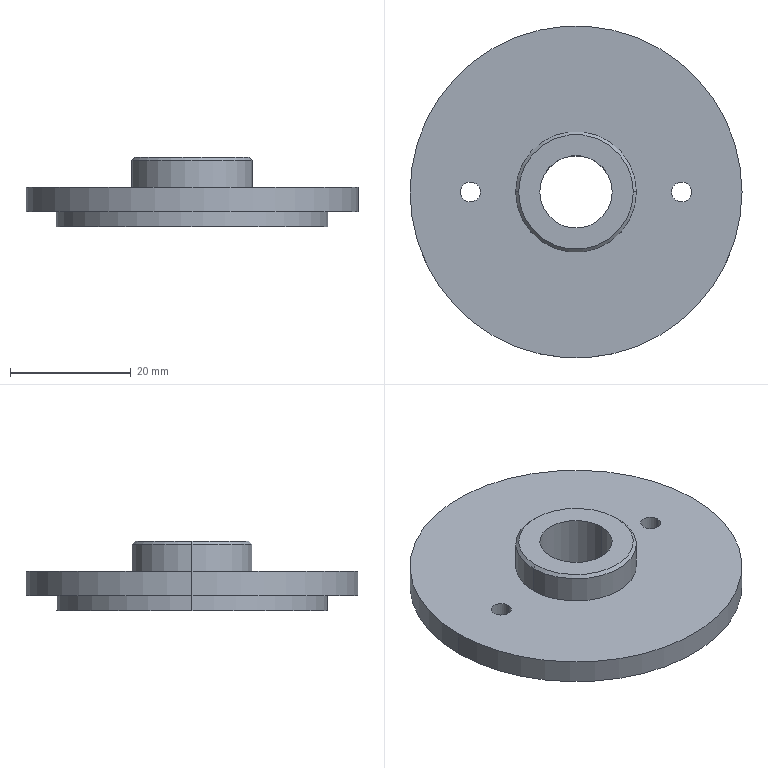Part | STEP file | PN_0098 tensioning part | 1 solid | 18 faces | box 55 x 55 x 11.5 mm | volume 13631 mm3 | cylinder 12 | plane 4 | cone 2 | commonest cylinder face diameters 3.3 x4 12 x2 20 x2 45 x2 55 x2
STEP:
#1=CARTESIAN_POINT('',(0.,0.,0.));
#2=DIRECTION('',(0.,0.,1.));
#3=DIRECTION('',(1.,0.,0.));
#4=AXIS2_PLACEMENT_3D('',#1,#2,#3);
#5=CARTESIAN_POINT('',(9.5,0.,9.));
#6=VERTEX_POINT('',#5);
#7=CARTESIAN_POINT('',(-9.5,0.,9.));
#8=VERTEX_POINT('',#7);
#9=CARTESIAN_POINT('',(0.,0.,9.));
#10=DIRECTION('',(0.,0.,1.));
#11=DIRECTION('',(1.,0.,0.));
#12=AXIS2_PLACEMENT_3D('',#9,#10,#11);
#13=CIRCLE('',#12,9.5);
#14=CARTESIAN_POINT('',(0.,0.,9.));
#15=DIRECTION('',(0.,0.,-1.));
#16=DIRECTION('',(-1.,0.,0.));
#17=AXIS2_PLACEMENT_3D('',#14,#15,#16);
#18=CONICAL_SURFACE('',#17,9.5,0.7854);
#19=CARTESIAN_POINT('',(3.142,0.));
#20=DIRECTION('',(-1.,0.));
#21=VECTOR('',#20,1.);
#22=LINE('',#19,#21);
#23=(GEOMETRIC_REPRESENTATION_CONTEXT(2)PARAMETRIC_REPRESENTATION_CONTEXT()REPRESENTATION_CONTEXT('',''));
#24=DEFINITIONAL_REPRESENTATION('',(#22),#23);
#25=PCURVE('',#18,#24);
#26=CARTESIAN_POINT('',(0.,0.,9.));
#27=DIRECTION('',(0.,0.,1.));
#28=DIRECTION('',(1.,0.,0.));
#29=AXIS2_PLACEMENT_3D('',#26,#27,#28);
#30=PLANE('',#29);
#31=CARTESIAN_POINT('',(0.,0.));
#32=DIRECTION('',(1.,0.));
#33=AXIS2_PLACEMENT_2D('',#31,#32);
#34=CIRCLE('',#33,9.5);
#35=(GEOMETRIC_REPRESENTATION_CONTEXT(2)PARAMETRIC_REPRESENTATION_CONTEXT()REPRESENTATION_CONTEXT('',''));
#36=DEFINITIONAL_REPRESENTATION('',(#34),#35);
#37=PCURVE('',#30,#36);
#38=SURFACE_CURVE('',#13,(#25,#37),.PCURVE_S1.);
#39=EDGE_CURVE('',#6,#8,#38,.T.);
#40=ORIENTED_EDGE('',*,*,#39,.F.);
#41=CARTESIAN_POINT('',(10.,0.,8.5));
#42=VERTEX_POINT('',#41);
#43=CARTESIAN_POINT('',(9.5,0.,9.));
#44=DIRECTION('',(0.7071,0.,-0.7071));
#45=VECTOR('',#44,1.);
#46=LINE('',#43,#45);
#47=CARTESIAN_POINT('',(3.142,0.));
#48=DIRECTION('',(0.,1.));
#49=VECTOR('',#48,1.);
#50=LINE('',#47,#49);
#51=(GEOMETRIC_REPRESENTATION_CONTEXT(2)PARAMETRIC_REPRESENTATION_CONTEXT()REPRESENTATION_CONTEXT('',''));
#52=DEFINITIONAL_REPRESENTATION('',(#50),#51);
#53=PCURVE('',#18,#52);
#54=CARTESIAN_POINT('',(0.,0.,9.));
#55=DIRECTION('',(0.,0.,-1.));
#56=DIRECTION('',(-1.,0.,0.));
#57=AXIS2_PLACEMENT_3D('',#54,#55,#56);
#58=CONICAL_SURFACE('',#57,9.5,0.7854);
#59=CARTESIAN_POINT('',(3.142,0.));
#60=DIRECTION('',(0.,1.));
#61=VECTOR('',#60,1.);
#62=LINE('',#59,#61);
#63=(GEOMETRIC_REPRESENTATION_CONTEXT(2)PARAMETRIC_REPRESENTATION_CONTEXT()REPRESENTATION_CONTEXT('',''));
#64=DEFINITIONAL_REPRESENTATION('',(#62),#63);
#65=PCURVE('',#58,#64);
#66=SURFACE_CURVE('',#46,(#53,#65),.PCURVE_S1.);
#67=EDGE_CURVE('',#6,#42,#66,.T.);
#68=ORIENTED_EDGE('',*,*,#67,.T.);
#69=CARTESIAN_POINT('',(-10.,0.,8.5));
#70=VERTEX_POINT('',#69);
#71=CARTESIAN_POINT('',(0.,0.,8.5));
#72=DIRECTION('',(0.,0.,-1.));
#73=DIRECTION('',(1.,0.,0.));
#74=AXIS2_PLACEMENT_3D('',#71,#72,#73);
#75=CIRCLE('',#74,10.);
#76=CARTESIAN_POINT('',(-3.142,0.5));
#77=DIRECTION('',(1.,0.));
#78=VECTOR('',#77,1.);
#79=LINE('',#76,#78);
#80=(GEOMETRIC_REPRESENTATION_CONTEXT(2)PARAMETRIC_REPRESENTATION_CONTEXT()REPRESENTATION_CONTEXT('',''));
#81=DEFINITIONAL_REPRESENTATION('',(#79),#80);
#82=PCURVE('',#18,#81);
#83=CARTESIAN_POINT('',(0.,0.,9.));
#84=DIRECTION('',(0.,0.,-1.));
#85=DIRECTION('',(-1.,0.,0.));
#86=AXIS2_PLACEMENT_3D('',#83,#84,#85);
#87=CYLINDRICAL_SURFACE('',#86,10.);
#88=CARTESIAN_POINT('',(-3.142,0.5));
#89=DIRECTION('',(1.,0.));
#90=VECTOR('',#89,1.);
#91=LINE('',#88,#90);
#92=(GEOMETRIC_REPRESENTATION_CONTEXT(2)PARAMETRIC_REPRESENTATION_CONTEXT()REPRESENTATION_CONTEXT('',''));
#93=DEFINITIONAL_REPRESENTATION('',(#91),#92);
#94=PCURVE('',#87,#93);
#95=SURFACE_CURVE('',#75,(#82,#94),.PCURVE_S1.);
#96=EDGE_CURVE('',#70,#42,#95,.T.);
#97=ORIENTED_EDGE('',*,*,#96,.F.);
#98=CARTESIAN_POINT('',(-9.5,0.,9.));
#99=DIRECTION('',(-0.7071,0.,-0.7071));
#100=VECTOR('',#99,1.);
#101=LINE('',#98,#100);
#102=CARTESIAN_POINT('',(0.,0.));
#103=DIRECTION('',(0.,1.));
#104=VECTOR('',#103,1.);
#105=LINE('',#102,#104);
#106=(GEOMETRIC_REPRESENTATION_CONTEXT(2)PARAMETRIC_REPRESENTATION_CONTEXT()REPRESENTATION_CONTEXT('',''));
#107=DEFINITIONAL_REPRESENTATION('',(#105),#106);
#108=PCURVE('',#18,#107);
#109=CARTESIAN_POINT('',(6.283,0.));
#110=DIRECTION('',(0.,1.));
#111=VECTOR('',#110,1.);
#112=LINE('',#109,#111);
#113=(GEOMETRIC_REPRESENTATION_CONTEXT(2)PARAMETRIC_REPRESENTATION_CONTEXT()REPRESENTATION_CONTEXT('',''));
#114=DEFINITIONAL_REPRESENTATION('',(#112),#113);
#115=PCURVE('',#58,#114);
#116=SURFACE_CURVE('',#101,(#108,#115),.PCURVE_S1.);
#117=EDGE_CURVE('',#8,#70,#116,.T.);
#118=ORIENTED_EDGE('',*,*,#117,.F.);
#119=EDGE_LOOP('',(#40,#68,#97,#118));
#120=FACE_BOUND('',#119,.T.);
#121=ADVANCED_FACE('',(#120),#18,.T.);
#122=CARTESIAN_POINT('',(-15.85,0.,-2.5));
#123=VERTEX_POINT('',#122);
#124=CARTESIAN_POINT('',(-15.85,0.,4.));
#125=VERTEX_POINT('',#124);
#126=CARTESIAN_POINT('',(-15.85,0.,4.));
#127=DIRECTION('',(0.,0.,1.));
#128=VECTOR('',#127,1.);
#129=LINE('',#126,#128);
#130=CARTESIAN_POINT('',(-17.5,0.,4.));
#131=DIRECTION('',(0.,0.,1.));
#132=DIRECTION('',(1.,0.,0.));
#133=AXIS2_PLACEMENT_3D('',#130,#131,#132);
#134=CYLINDRICAL_SURFACE('',#133,1.65);
#135=CARTESIAN_POINT('',(6.283,0.));
#136=DIRECTION('',(0.,1.));
#137=VECTOR('',#136,1.);
#138=LINE('',#135,#137);
#139=(GEOMETRIC_REPRESENTATION_CONTEXT(2)PARAMETRIC_REPRESENTATION_CONTEXT()REPRESENTATION_CONTEXT('',''));
#140=DEFINITIONAL_REPRESENTATION('',(#138),#139);
#141=PCURVE('',#134,#140);
#142=CARTESIAN_POINT('',(-17.5,0.,4.));
#143=DIRECTION('',(0.,0.,1.));
#144=DIRECTION('',(1.,0.,0.));
#145=AXIS2_PLACEMENT_3D('',#142,#143,#144);
#146=CYLINDRICAL_SURFACE('',#145,1.65);
#147=CARTESIAN_POINT('',(0.,0.));
#148=DIRECTION('',(0.,1.));
#149=VECTOR('',#148,1.);
#150=LINE('',#147,#149);
#151=(GEOMETRIC_REPRESENTATION_CONTEXT(2)PARAMETRIC_REPRESENTATION_CONTEXT()REPRESENTATION_CONTEXT('',''));
#152=DEFINITIONAL_REPRESENTATION('',(#150),#151);
#153=PCURVE('',#146,#152);
#154=SURFACE_CURVE('',#129,(#141,#153),.PCURVE_S1.);
#155=EDGE_CURVE('',#123,#125,#154,.T.);
#156=ORIENTED_EDGE('',*,*,#155,.T.);
#157=CARTESIAN_POINT('',(-19.15,0.,4.));
#158=VERTEX_POINT('',#157);
#159=CARTESIAN_POINT('',(-17.5,0.,4.));
#160=DIRECTION('',(0.,0.,1.));
#161=DIRECTION('',(1.,0.,0.));
#162=AXIS2_PLACEMENT_3D('',#159,#160,#161);
#163=CIRCLE('',#162,1.65);
#164=CARTESIAN_POINT('',(0.,0.));
#165=DIRECTION('',(1.,0.));
#166=VECTOR('',#165,1.);
#167=LINE('',#164,#166);
#168=(GEOMETRIC_REPRESENTATION_CONTEXT(2)PARAMETRIC_REPRESENTATION_CONTEXT()REPRESENTATION_CONTEXT('',''));
#169=DEFINITIONAL_REPRESENTATION('',(#167),#168);
#170=PCURVE('',#134,#169);
#171=CARTESIAN_POINT('',(0.,0.,4.));
#172=DIRECTION('',(0.,0.,1.));
#173=DIRECTION('',(1.,0.,0.));
#174=AXIS2_PLACEMENT_3D('',#171,#172,#173);
#175=PLANE('',#174);
#176=CARTESIAN_POINT('',(-17.5,0.));
#177=DIRECTION('',(1.,0.));
#178=AXIS2_PLACEMENT_2D('',#176,#177);
#179=CIRCLE('',#178,1.65);
#180=(GEOMETRIC_REPRESENTATION_CONTEXT(2)PARAMETRIC_REPRESENTATION_CONTEXT()REPRESENTATION_CONTEXT('',''));
#181=DEFINITIONAL_REPRESENTATION('',(#179),#180);
#182=PCURVE('',#175,#181);
#183=SURFACE_CURVE('',#163,(#170,#182),.PCURVE_S1.);
#184=EDGE_CURVE('',#158,#125,#183,.T.);
#185=ORIENTED_EDGE('',*,*,#184,.F.);
#186=CARTESIAN_POINT('',(-19.15,0.,-2.5));
#187=VERTEX_POINT('',#186);
#188=CARTESIAN_POINT('',(-19.15,0.,4.));
#189=DIRECTION('',(0.,0.,1.));
#190=VECTOR('',#189,1.);
#191=LINE('',#188,#190);
#192=CARTESIAN_POINT('',(3.142,0.));
#193=DIRECTION('',(0.,1.));
#194=VECTOR('',#193,1.);
#195=LINE('',#192,#194);
#196=(GEOMETRIC_REPRESENTATION_CONTEXT(2)PARAMETRIC_REPRESENTATION_CONTEXT()REPRESENTATION_CONTEXT('',''));
#197=DEFINITIONAL_REPRESENTATION('',(#195),#196);
#198=PCURVE('',#134,#197);
#199=CARTESIAN_POINT('',(3.142,0.));
#200=DIRECTION('',(0.,1.));
#201=VECTOR('',#200,1.);
#202=LINE('',#199,#201);
#203=(GEOMETRIC_REPRESENTATION_CONTEXT(2)PARAMETRIC_REPRESENTATION_CONTEXT()REPRESENTATION_CONTEXT('',''));
#204=DEFINITIONAL_REPRESENTATION('',(#202),#203);
#205=PCURVE('',#146,#204);
#206=SURFACE_CURVE('',#191,(#198,#205),.PCURVE_S1.);
#207=EDGE_CURVE('',#187,#158,#206,.T.);
#208=ORIENTED_EDGE('',*,*,#207,.F.);
#209=CARTESIAN_POINT('',(-17.5,0.,-2.5));
#210=DIRECTION('',(0.,0.,1.));
#211=DIRECTION('',(1.,0.,0.));
#212=AXIS2_PLACEMENT_3D('',#209,#210,#211);
#213=CIRCLE('',#212,1.65);
#214=CARTESIAN_POINT('',(0.,-6.5));
#215=DIRECTION('',(1.,0.));
#216=VECTOR('',#215,1.);
#217=LINE('',#214,#216);
#218=(GEOMETRIC_REPRESENTATION_CONTEXT(2)PARAMETRIC_REPRESENTATION_CONTEXT()REPRESENTATION_CONTEXT('',''));
#219=DEFINITIONAL_REPRESENTATION('',(#217),#218);
#220=PCURVE('',#134,#219);
#221=CARTESIAN_POINT('',(0.,0.,-2.5));
#222=DIRECTION('',(0.,0.,-1.));
#223=DIRECTION('',(-1.,0.,0.));
#224=AXIS2_PLACEMENT_3D('',#221,#222,#223);
#225=PLANE('',#224);
#226=CARTESIAN_POINT('',(15.85,0.));
#227=CARTESIAN_POINT('',(15.85,2.858));
#228=CARTESIAN_POINT('',(18.325,1.429));
#229=CARTESIAN_POINT('',(20.8,0.));
#230=CARTESIAN_POINT('',(18.325,-1.429));
#231=CARTESIAN_POINT('',(15.85,-2.858));
#232=CARTESIAN_POINT('',(15.85,0.));
#233=(BOUNDED_CURVE()B_SPLINE_CURVE(2,(#226,#227,#228,#229,#230,#231,#232),.UNSPECIFIED.,.T.,.F.)B_SPLINE_CURVE_WITH_KNOTS((1,2,2,2,2,1),(-2.094,0.,2.094,4.189,6.283,8.378),.UNSPECIFIED.)CURVE()GEOMETRIC_REPRESENTATION_ITEM()RATIONAL_B_SPLINE_CURVE((1.,0.5,1.,0.5,1.,0.5,1.))REPRESENTATION_ITEM(''));
#234=(GEOMETRIC_REPRESENTATION_CONTEXT(2)PARAMETRIC_REPRESENTATION_CONTEXT()REPRESENTATION_CONTEXT('',''));
#235=DEFINITIONAL_REPRESENTATION('',(#233),#234);
#236=PCURVE('',#225,#235);
#237=SURFACE_CURVE('',#213,(#220,#236),.PCURVE_S1.);
#238=EDGE_CURVE('',#187,#123,#237,.T.);
#239=ORIENTED_EDGE('',*,*,#238,.T.);
#240=EDGE_LOOP('',(#156,#185,#208,#239));
#241=FACE_BOUND('',#240,.F.);
#242=ADVANCED_FACE('',(#241),#134,.F.);
#243=CARTESIAN_POINT('',(19.15,0.,-2.5));
#244=VERTEX_POINT('',#243);
#245=CARTESIAN_POINT('',(19.15,0.,4.));
#246=VERTEX_POINT('',#245);
#247=CARTESIAN_POINT('',(19.15,0.,4.));
#248=DIRECTION('',(0.,0.,1.));
#249=VECTOR('',#248,1.);
#250=LINE('',#247,#249);
#251=CARTESIAN_POINT('',(17.5,0.,4.));
#252=DIRECTION('',(0.,0.,1.));
#253=DIRECTION('',(1.,0.,0.));
#254=AXIS2_PLACEMENT_3D('',#251,#252,#253);
#255=CYLINDRICAL_SURFACE('',#254,1.65);
#256=CARTESIAN_POINT('',(6.283,0.));
#257=DIRECTION('',(0.,1.));
#258=VECTOR('',#257,1.);
#259=LINE('',#256,#258);
#260=(GEOMETRIC_REPRESENTATION_CONTEXT(2)PARAMETRIC_REPRESENTATION_CONTEXT()REPRESENTATION_CONTEXT('',''));
#261=DEFINITIONAL_REPRESENTATION('',(#259),#260);
#262=PCURVE('',#255,#261);
#263=CARTESIAN_POINT('',(17.5,0.,4.));
#264=DIRECTION('',(0.,0.,1.));
#265=DIRECTION('',(1.,0.,0.));
#266=AXIS2_PLACEMENT_3D('',#263,#264,#265);
#267=CYLINDRICAL_SURFACE('',#266,1.65);
#268=CARTESIAN_POINT('',(0.,0.));
#269=DIRECTION('',(0.,1.));
#270=VECTOR('',#269,1.);
#271=LINE('',#268,#270);
#272=(GEOMETRIC_REPRESENTATION_CONTEXT(2)PARAMETRIC_REPRESENTATION_CONTEXT()REPRESENTATION_CONTEXT('',''));
#273=DEFINITIONAL_REPRESENTATION('',(#271),#272);
#274=PCURVE('',#267,#273);
#275=SURFACE_CURVE('',#250,(#262,#274),.PCURVE_S1.);
#276=EDGE_CURVE('',#244,#246,#275,.T.);
#277=ORIENTED_EDGE('',*,*,#276,.T.);
#278=CARTESIAN_POINT('',(15.85,0.,4.));
#279=VERTEX_POINT('',#278);
#280=CARTESIAN_POINT('',(17.5,0.,4.));
#281=DIRECTION('',(0.,0.,1.));
#282=DIRECTION('',(1.,0.,0.));
#283=AXIS2_PLACEMENT_3D('',#280,#281,#282);
#284=CIRCLE('',#283,1.65);
#285=CARTESIAN_POINT('',(0.,0.));
#286=DIRECTION('',(1.,0.));
#287=VECTOR('',#286,1.);
#288=LINE('',#285,#287);
#289=(GEOMETRIC_REPRESENTATION_CONTEXT(2)PARAMETRIC_REPRESENTATION_CONTEXT()REPRESENTATION_CONTEXT('',''));
#290=DEFINITIONAL_REPRESENTATION('',(#288),#289);
#291=PCURVE('',#255,#290);
#292=CARTESIAN_POINT('',(17.5,0.));
#293=DIRECTION('',(1.,0.));
#294=AXIS2_PLACEMENT_2D('',#292,#293);
#295=CIRCLE('',#294,1.65);
#296=(GEOMETRIC_REPRESENTATION_CONTEXT(2)PARAMETRIC_REPRESENTATION_CONTEXT()REPRESENTATION_CONTEXT('',''));
#297=DEFINITIONAL_REPRESENTATION('',(#295),#296);
#298=PCURVE('',#175,#297);
#299=SURFACE_CURVE('',#284,(#291,#298),.PCURVE_S1.);
#300=EDGE_CURVE('',#279,#246,#299,.T.);
#301=ORIENTED_EDGE('',*,*,#300,.F.);
#302=CARTESIAN_POINT('',(15.85,0.,-2.5));
#303=VERTEX_POINT('',#302);
#304=CARTESIAN_POINT('',(15.85,0.,4.));
#305=DIRECTION('',(0.,0.,1.));
#306=VECTOR('',#305,1.);
#307=LINE('',#304,#306);
#308=CARTESIAN_POINT('',(3.142,0.));
#309=DIRECTION('',(0.,1.));
#310=VECTOR('',#309,1.);
#311=LINE('',#308,#310);
#312=(GEOMETRIC_REPRESENTATION_CONTEXT(2)PARAMETRIC_REPRESENTATION_CONTEXT()REPRESENTATION_CONTEXT('',''));
#313=DEFINITIONAL_REPRESENTATION('',(#311),#312);
#314=PCURVE('',#255,#313);
#315=CARTESIAN_POINT('',(3.142,0.));
#316=DIRECTION('',(0.,1.));
#317=VECTOR('',#316,1.);
#318=LINE('',#315,#317);
#319=(GEOMETRIC_REPRESENTATION_CONTEXT(2)PARAMETRIC_REPRESENTATION_CONTEXT()REPRESENTATION_CONTEXT('',''));
#320=DEFINITIONAL_REPRESENTATION('',(#318),#319);
#321=PCURVE('',#267,#320);
#322=SURFACE_CURVE('',#307,(#314,#321),.PCURVE_S1.);
#323=EDGE_CURVE('',#303,#279,#322,.T.);
#324=ORIENTED_EDGE('',*,*,#323,.F.);
#325=CARTESIAN_POINT('',(17.5,0.,-2.5));
#326=DIRECTION('',(0.,0.,1.));
#327=DIRECTION('',(1.,0.,0.));
#328=AXIS2_PLACEMENT_3D('',#325,#326,#327);
#329=CIRCLE('',#328,1.65);
#330=CARTESIAN_POINT('',(0.,-6.5));
#331=DIRECTION('',(1.,0.));
#332=VECTOR('',#331,1.);
#333=LINE('',#330,#332);
#334=(GEOMETRIC_REPRESENTATION_CONTEXT(2)PARAMETRIC_REPRESENTATION_CONTEXT()REPRESENTATION_CONTEXT('',''));
#335=DEFINITIONAL_REPRESENTATION('',(#333),#334);
#336=PCURVE('',#255,#335);
#337=CARTESIAN_POINT('',(-19.15,0.));
#338=CARTESIAN_POINT('',(-19.15,2.858));
#339=CARTESIAN_POINT('',(-16.675,1.429));
#340=CARTESIAN_POINT('',(-14.2,0.));
#341=CARTESIAN_POINT('',(-16.675,-1.429));
#342=CARTESIAN_POINT('',(-19.15,-2.858));
#343=CARTESIAN_POINT('',(-19.15,0.));
#344=(BOUNDED_CURVE()B_SPLINE_CURVE(2,(#337,#338,#339,#340,#341,#342,#343),.UNSPECIFIED.,.T.,.F.)B_SPLINE_CURVE_WITH_KNOTS((1,2,2,2,2,1),(-2.094,0.,2.094,4.189,6.283,8.378),.UNSPECIFIED.)CURVE()GEOMETRIC_REPRESENTATION_ITEM()RATIONAL_B_SPLINE_CURVE((1.,0.5,1.,0.5,1.,0.5,1.))REPRESENTATION_ITEM(''));
#345=(GEOMETRIC_REPRESENTATION_CONTEXT(2)PARAMETRIC_REPRESENTATION_CONTEXT()REPRESENTATION_CONTEXT('',''));
#346=DEFINITIONAL_REPRESENTATION('',(#344),#345);
#347=PCURVE('',#225,#346);
#348=SURFACE_CURVE('',#329,(#336,#347),.PCURVE_S1.);
#349=EDGE_CURVE('',#303,#244,#348,.T.);
#350=ORIENTED_EDGE('',*,*,#349,.T.);
#351=EDGE_LOOP('',(#277,#301,#324,#350));
#352=FACE_BOUND('',#351,.F.);
#353=ADVANCED_FACE('',(#352),#255,.F.);
#354=CARTESIAN_POINT('',(-22.5,0.,-2.5));
#355=VERTEX_POINT('',#354);
#356=CARTESIAN_POINT('',(22.5,0.,-2.5));
#357=VERTEX_POINT('',#356);
#358=CARTESIAN_POINT('',(0.,0.,-2.5));
#359=DIRECTION('',(0.,0.,-1.));
#360=DIRECTION('',(-1.,0.,0.));
#361=AXIS2_PLACEMENT_3D('',#358,#359,#360);
#362=CIRCLE('',#361,22.5);
#363=CARTESIAN_POINT('',(0.,0.,-2.5));
#364=DIRECTION('',(0.,0.,1.));
#365=DIRECTION('',(1.,0.,0.));
#366=AXIS2_PLACEMENT_3D('',#363,#364,#365);
#367=CYLINDRICAL_SURFACE('',#366,22.5);
#368=CARTESIAN_POINT('',(3.142,0.));
#369=DIRECTION('',(-1.,0.));
#370=VECTOR('',#369,1.);
#371=LINE('',#368,#370);
#372=(GEOMETRIC_REPRESENTATION_CONTEXT(2)PARAMETRIC_REPRESENTATION_CONTEXT()REPRESENTATION_CONTEXT('',''));
#373=DEFINITIONAL_REPRESENTATION('',(#371),#372);
#374=PCURVE('',#367,#373);
#375=CARTESIAN_POINT('',(0.,0.));
#376=DIRECTION('',(1.,0.));
#377=AXIS2_PLACEMENT_2D('',#375,#376);
#378=CIRCLE('',#377,22.5);
#379=(GEOMETRIC_REPRESENTATION_CONTEXT(2)PARAMETRIC_REPRESENTATION_CONTEXT()REPRESENTATION_CONTEXT('',''));
#380=DEFINITIONAL_REPRESENTATION('',(#378),#379);
#381=PCURVE('',#225,#380);
#382=SURFACE_CURVE('',#362,(#374,#381),.PCURVE_S1.);
#383=EDGE_CURVE('',#355,#357,#382,.T.);
#384=ORIENTED_EDGE('',*,*,#383,.F.);
#385=CARTESIAN_POINT('',(-22.5,0.,0.));
#386=VERTEX_POINT('',#385);
#387=CARTESIAN_POINT('',(-22.5,0.,-2.5));
#388=DIRECTION('',(0.,0.,1.));
#389=VECTOR('',#388,1.);
#390=LINE('',#387,#389);
#391=CARTESIAN_POINT('',(3.142,0.));
#392=DIRECTION('',(0.,1.));
#393=VECTOR('',#392,1.);
#394=LINE('',#391,#393);
#395=(GEOMETRIC_REPRESENTATION_CONTEXT(2)PARAMETRIC_REPRESENTATION_CONTEXT()REPRESENTATION_CONTEXT('',''));
#396=DEFINITIONAL_REPRESENTATION('',(#394),#395);
#397=PCURVE('',#367,#396);
#398=CARTESIAN_POINT('',(0.,0.,-2.5));
#399=DIRECTION('',(0.,0.,1.));
#400=DIRECTION('',(1.,0.,0.));
#401=AXIS2_PLACEMENT_3D('',#398,#399,#400);
#402=CYLINDRICAL_SURFACE('',#401,22.5);
#403=CARTESIAN_POINT('',(3.142,0.));
#404=DIRECTION('',(0.,1.));
#405=VECTOR('',#404,1.);
#406=LINE('',#403,#405);
#407=(GEOMETRIC_REPRESENTATION_CONTEXT(2)PARAMETRIC_REPRESENTATION_CONTEXT()REPRESENTATION_CONTEXT('',''));
#408=DEFINITIONAL_REPRESENTATION('',(#406),#407);
#409=PCURVE('',#402,#408);
#410=SURFACE_CURVE('',#390,(#397,#409),.PCURVE_S1.);
#411=EDGE_CURVE('',#355,#386,#410,.T.);
#412=ORIENTED_EDGE('',*,*,#411,.T.);
#413=CARTESIAN_POINT('',(22.5,0.,0.));
#414=VERTEX_POINT('',#413);
#415=CARTESIAN_POINT('',(0.,0.,0.));
#416=DIRECTION('',(0.,0.,-1.));
#417=DIRECTION('',(1.,0.,0.));
#418=AXIS2_PLACEMENT_3D('',#415,#416,#417);
#419=CIRCLE('',#418,22.5);
#420=CARTESIAN_POINT('',(6.283,2.5));
#421=DIRECTION('',(-1.,0.));
#422=VECTOR('',#421,1.);
#423=LINE('',#420,#422);
#424=(GEOMETRIC_REPRESENTATION_CONTEXT(2)PARAMETRIC_REPRESENTATION_CONTEXT()REPRESENTATION_CONTEXT('',''));
#425=DEFINITIONAL_REPRESENTATION('',(#423),#424);
#426=PCURVE('',#367,#425);
#427=CARTESIAN_POINT('',(0.,0.,0.));
#428=DIRECTION('',(0.,0.,1.));
#429=DIRECTION('',(1.,0.,0.));
#430=AXIS2_PLACEMENT_3D('',#427,#428,#429);
#431=PLANE('',#430);
#432=CARTESIAN_POINT('',(22.5,0.));
#433=CARTESIAN_POINT('',(22.5,-38.971));
#434=CARTESIAN_POINT('',(-11.25,-19.486));
#435=CARTESIAN_POINT('',(-45.,0.));
#436=CARTESIAN_POINT('',(-11.25,19.486));
#437=CARTESIAN_POINT('',(22.5,38.971));
#438=CARTESIAN_POINT('',(22.5,0.));
#439=(BOUNDED_CURVE()B_SPLINE_CURVE(2,(#432,#433,#434,#435,#436,#437,#438),.UNSPECIFIED.,.T.,.F.)B_SPLINE_CURVE_WITH_KNOTS((1,2,2,2,2,1),(-2.094,0.,2.094,4.189,6.283,8.378),.UNSPECIFIED.)CURVE()GEOMETRIC_REPRESENTATION_ITEM()RATIONAL_B_SPLINE_CURVE((1.,0.5,1.,0.5,1.,0.5,1.))REPRESENTATION_ITEM(''));
#440=(GEOMETRIC_REPRESENTATION_CONTEXT(2)PARAMETRIC_REPRESENTATION_CONTEXT()REPRESENTATION_CONTEXT('',''));
#441=DEFINITIONAL_REPRESENTATION('',(#439),#440);
#442=PCURVE('',#431,#441);
#443=SURFACE_CURVE('',#419,(#426,#442),.PCURVE_S1.);
#444=EDGE_CURVE('',#386,#414,#443,.T.);
#445=ORIENTED_EDGE('',*,*,#444,.T.);
#446=CARTESIAN_POINT('',(22.5,0.,-2.5));
#447=DIRECTION('',(0.,0.,1.));
#448=VECTOR('',#447,1.);
#449=LINE('',#446,#448);
#450=CARTESIAN_POINT('',(0.,0.));
#451=DIRECTION('',(0.,1.));
#452=VECTOR('',#451,1.);
#453=LINE('',#450,#452);
#454=(GEOMETRIC_REPRESENTATION_CONTEXT(2)PARAMETRIC_REPRESENTATION_CONTEXT()REPRESENTATION_CONTEXT('',''));
#455=DEFINITIONAL_REPRESENTATION('',(#453),#454);
#456=PCURVE('',#367,#455);
#457=CARTESIAN_POINT('',(6.283,0.));
#458=DIRECTION('',(0.,1.));
#459=VECTOR('',#458,1.);
#460=LINE('',#457,#459);
#461=(GEOMETRIC_REPRESENTATION_CONTEXT(2)PARAMETRIC_REPRESENTATION_CONTEXT()REPRESENTATION_CONTEXT('',''));
#462=DEFINITIONAL_REPRESENTATION('',(#460),#461);
#463=PCURVE('',#402,#462);
#464=SURFACE_CURVE('',#449,(#456,#463),.PCURVE_S1.);
#465=EDGE_CURVE('',#357,#414,#464,.T.);
#466=ORIENTED_EDGE('',*,*,#465,.F.);
#467=EDGE_LOOP('',(#384,#412,#445,#466));
#468=FACE_BOUND('',#467,.T.);
#469=ADVANCED_FACE('',(#468),#367,.T.);
#470=ORIENTED_EDGE('',*,*,#96,.T.);
#471=CARTESIAN_POINT('',(10.,0.,4.));
#472=VERTEX_POINT('',#471);
#473=CARTESIAN_POINT('',(10.,0.,9.));
#474=DIRECTION('',(0.,0.,-1.));
#475=VECTOR('',#474,1.);
#476=LINE('',#473,#475);
#477=CARTESIAN_POINT('',(3.142,0.));
#478=DIRECTION('',(0.,1.));
#479=VECTOR('',#478,1.);
#480=LINE('',#477,#479);
#481=(GEOMETRIC_REPRESENTATION_CONTEXT(2)PARAMETRIC_REPRESENTATION_CONTEXT()REPRESENTATION_CONTEXT('',''));
#482=DEFINITIONAL_REPRESENTATION('',(#480),#481);
#483=PCURVE('',#87,#482);
#484=CARTESIAN_POINT('',(0.,0.,9.));
#485=DIRECTION('',(0.,0.,-1.));
#486=DIRECTION('',(-1.,0.,0.));
#487=AXIS2_PLACEMENT_3D('',#484,#485,#486);
#488=CYLINDRICAL_SURFACE('',#487,10.);
#489=CARTESIAN_POINT('',(3.142,0.));
#490=DIRECTION('',(0.,1.));
#491=VECTOR('',#490,1.);
#492=LINE('',#489,#491);
#493=(GEOMETRIC_REPRESENTATION_CONTEXT(2)PARAMETRIC_REPRESENTATION_CONTEXT()REPRESENTATION_CONTEXT('',''));
#494=DEFINITIONAL_REPRESENTATION('',(#492),#493);
#495=PCURVE('',#488,#494);
#496=SURFACE_CURVE('',#476,(#483,#495),.PCURVE_S1.);
#497=EDGE_CURVE('',#42,#472,#496,.T.);
#498=ORIENTED_EDGE('',*,*,#497,.T.);
#499=CARTESIAN_POINT('',(-10.,0.,4.));
#500=VERTEX_POINT('',#499);
#501=CARTESIAN_POINT('',(0.,0.,4.));
#502=DIRECTION('',(0.,0.,1.));
#503=DIRECTION('',(1.,0.,0.));
#504=AXIS2_PLACEMENT_3D('',#501,#502,#503);
#505=CIRCLE('',#504,10.);
#506=CARTESIAN_POINT('',(3.142,5.));
#507=DIRECTION('',(-1.,0.));
#508=VECTOR('',#507,1.);
#509=LINE('',#506,#508);
#510=(GEOMETRIC_REPRESENTATION_CONTEXT(2)PARAMETRIC_REPRESENTATION_CONTEXT()REPRESENTATION_CONTEXT('',''));
#511=DEFINITIONAL_REPRESENTATION('',(#509),#510);
#512=PCURVE('',#87,#511);
#513=CARTESIAN_POINT('',(0.,0.));
#514=DIRECTION('',(1.,0.));
#515=AXIS2_PLACEMENT_2D('',#513,#514);
#516=CIRCLE('',#515,10.);
#517=(GEOMETRIC_REPRESENTATION_CONTEXT(2)PARAMETRIC_REPRESENTATION_CONTEXT()REPRESENTATION_CONTEXT('',''));
#518=DEFINITIONAL_REPRESENTATION('',(#516),#517);
#519=PCURVE('',#175,#518);
#520=SURFACE_CURVE('',#505,(#512,#519),.PCURVE_S1.);
#521=EDGE_CURVE('',#472,#500,#520,.T.);
#522=ORIENTED_EDGE('',*,*,#521,.T.);
#523=CARTESIAN_POINT('',(-10.,0.,9.));
#524=DIRECTION('',(0.,0.,-1.));
#525=VECTOR('',#524,1.);
#526=LINE('',#523,#525);
#527=CARTESIAN_POINT('',(0.,0.));
#528=DIRECTION('',(0.,1.));
#529=VECTOR('',#528,1.);
#530=LINE('',#527,#529);
#531=(GEOMETRIC_REPRESENTATION_CONTEXT(2)PARAMETRIC_REPRESENTATION_CONTEXT()REPRESENTATION_CONTEXT('',''));
#532=DEFINITIONAL_REPRESENTATION('',(#530),#531);
#533=PCURVE('',#87,#532);
#534=CARTESIAN_POINT('',(6.283,0.));
#535=DIRECTION('',(0.,1.));
#536=VECTOR('',#535,1.);
#537=LINE('',#534,#536);
#538=(GEOMETRIC_REPRESENTATION_CONTEXT(2)PARAMETRIC_REPRESENTATION_CONTEXT()REPRESENTATION_CONTEXT('',''));
#539=DEFINITIONAL_REPRESENTATION('',(#537),#538);
#540=PCURVE('',#488,#539);
#541=SURFACE_CURVE('',#526,(#533,#540),.PCURVE_S1.);
#542=EDGE_CURVE('',#70,#500,#541,.T.);
#543=ORIENTED_EDGE('',*,*,#542,.F.);
#544=EDGE_LOOP('',(#470,#498,#522,#543));
#545=FACE_BOUND('',#544,.T.);
#546=ADVANCED_FACE('',(#545),#87,.T.);
#547=CARTESIAN_POINT('',(-6.,0.,9.));
#548=VERTEX_POINT('',#547);
#549=CARTESIAN_POINT('',(-6.,0.,-2.5));
#550=VERTEX_POINT('',#549);
#551=CARTESIAN_POINT('',(-6.,0.,4.));
#552=DIRECTION('',(0.,0.,-1.));
#553=VECTOR('',#552,1.);
#554=LINE('',#551,#553);
#555=CARTESIAN_POINT('',(0.,0.,4.));
#556=DIRECTION('',(0.,0.,-1.));
#557=DIRECTION('',(-1.,0.,0.));
#558=AXIS2_PLACEMENT_3D('',#555,#556,#557);
#559=CYLINDRICAL_SURFACE('',#558,6.);
#560=CARTESIAN_POINT('',(6.283,0.));
#561=DIRECTION('',(0.,1.));
#562=VECTOR('',#561,1.);
#563=LINE('',#560,#562);
#564=(GEOMETRIC_REPRESENTATION_CONTEXT(2)PARAMETRIC_REPRESENTATION_CONTEXT()REPRESENTATION_CONTEXT('',''));
#565=DEFINITIONAL_REPRESENTATION('',(#563),#564);
#566=PCURVE('',#559,#565);
#567=CARTESIAN_POINT('',(0.,0.,4.));
#568=DIRECTION('',(0.,0.,-1.));
#569=DIRECTION('',(-1.,0.,0.));
#570=AXIS2_PLACEMENT_3D('',#567,#568,#569);
#571=CYLINDRICAL_SURFACE('',#570,6.);
#572=CARTESIAN_POINT('',(0.,0.));
#573=DIRECTION('',(0.,1.));
#574=VECTOR('',#573,1.);
#575=LINE('',#572,#574);
#576=(GEOMETRIC_REPRESENTATION_CONTEXT(2)PARAMETRIC_REPRESENTATION_CONTEXT()REPRESENTATION_CONTEXT('',''));
#577=DEFINITIONAL_REPRESENTATION('',(#575),#576);
#578=PCURVE('',#571,#577);
#579=SURFACE_CURVE('',#554,(#566,#578),.PCURVE_S1.);
#580=EDGE_CURVE('',#548,#550,#579,.T.);
#581=ORIENTED_EDGE('',*,*,#580,.T.);
#582=CARTESIAN_POINT('',(6.,0.,-2.5));
#583=VERTEX_POINT('',#582);
#584=CARTESIAN_POINT('',(0.,0.,-2.5));
#585=DIRECTION('',(0.,0.,-1.));
#586=DIRECTION('',(-1.,0.,0.));
#587=AXIS2_PLACEMENT_3D('',#584,#585,#586);
#588=CIRCLE('',#587,6.);
#589=CARTESIAN_POINT('',(0.,6.5));
#590=DIRECTION('',(1.,0.));
#591=VECTOR('',#590,1.);
#592=LINE('',#589,#591);
#593=(GEOMETRIC_REPRESENTATION_CONTEXT(2)PARAMETRIC_REPRESENTATION_CONTEXT()REPRESENTATION_CONTEXT('',''));
#594=DEFINITIONAL_REPRESENTATION('',(#592),#593);
#595=PCURVE('',#559,#594);
#596=CARTESIAN_POINT('',(0.,0.));
#597=DIRECTION('',(1.,0.));
#598=AXIS2_PLACEMENT_2D('',#596,#597);
#599=CIRCLE('',#598,6.);
#600=(GEOMETRIC_REPRESENTATION_CONTEXT(2)PARAMETRIC_REPRESENTATION_CONTEXT()REPRESENTATION_CONTEXT('',''));
#601=DEFINITIONAL_REPRESENTATION('',(#599),#600);
#602=PCURVE('',#225,#601);
#603=SURFACE_CURVE('',#588,(#595,#602),.PCURVE_S1.);
#604=EDGE_CURVE('',#583,#550,#603,.T.);
#605=ORIENTED_EDGE('',*,*,#604,.F.);
#606=CARTESIAN_POINT('',(6.,0.,9.));
#607=VERTEX_POINT('',#606);
#608=CARTESIAN_POINT('',(6.,0.,4.));
#609=DIRECTION('',(0.,0.,-1.));
#610=VECTOR('',#609,1.);
#611=LINE('',#608,#610);
#612=CARTESIAN_POINT('',(3.142,0.));
#613=DIRECTION('',(0.,1.));
#614=VECTOR('',#613,1.);
#615=LINE('',#612,#614);
#616=(GEOMETRIC_REPRESENTATION_CONTEXT(2)PARAMETRIC_REPRESENTATION_CONTEXT()REPRESENTATION_CONTEXT('',''));
#617=DEFINITIONAL_REPRESENTATION('',(#615),#616);
#618=PCURVE('',#559,#617);
#619=CARTESIAN_POINT('',(3.142,0.));
#620=DIRECTION('',(0.,1.));
#621=VECTOR('',#620,1.);
#622=LINE('',#619,#621);
#623=(GEOMETRIC_REPRESENTATION_CONTEXT(2)PARAMETRIC_REPRESENTATION_CONTEXT()REPRESENTATION_CONTEXT('',''));
#624=DEFINITIONAL_REPRESENTATION('',(#622),#623);
#625=PCURVE('',#571,#624);
#626=SURFACE_CURVE('',#611,(#618,#625),.PCURVE_S1.);
#627=EDGE_CURVE('',#607,#583,#626,.T.);
#628=ORIENTED_EDGE('',*,*,#627,.F.);
#629=CARTESIAN_POINT('',(0.,0.,9.));
#630=DIRECTION('',(0.,0.,1.));
#631=DIRECTION('',(1.,0.,0.));
#632=AXIS2_PLACEMENT_3D('',#629,#630,#631);
#633=CIRCLE('',#632,6.);
#634=CARTESIAN_POINT('',(9.425,-5.));
#635=DIRECTION('',(-1.,0.));
#636=VECTOR('',#635,1.);
#637=LINE('',#634,#636);
#638=(GEOMETRIC_REPRESENTATION_CONTEXT(2)PARAMETRIC_REPRESENTATION_CONTEXT()REPRESENTATION_CONTEXT('',''));
#639=DEFINITIONAL_REPRESENTATION('',(#637),#638);
#640=PCURVE('',#559,#639);
#641=CARTESIAN_POINT('',(0.,0.));
#642=DIRECTION('',(1.,0.));
#643=AXIS2_PLACEMENT_2D('',#641,#642);
#644=CIRCLE('',#643,6.);
#645=(GEOMETRIC_REPRESENTATION_CONTEXT(2)PARAMETRIC_REPRESENTATION_CONTEXT()REPRESENTATION_CONTEXT('',''));
#646=DEFINITIONAL_REPRESENTATION('',(#644),#645);
#647=PCURVE('',#30,#646);
#648=SURFACE_CURVE('',#633,(#640,#647),.PCURVE_S1.);
#649=EDGE_CURVE('',#548,#607,#648,.T.);
#650=ORIENTED_EDGE('',*,*,#649,.F.);
#651=EDGE_LOOP('',(#581,#605,#628,#650));
#652=FACE_BOUND('',#651,.F.);
#653=ADVANCED_FACE('',(#652),#559,.F.);
#654=CARTESIAN_POINT('',(27.5,0.,4.));
#655=VERTEX_POINT('',#654);
#656=CARTESIAN_POINT('',(-27.5,0.,4.));
#657=VERTEX_POINT('',#656);
#658=CARTESIAN_POINT('',(0.,0.,4.));
#659=DIRECTION('',(0.,0.,1.));
#660=DIRECTION('',(1.,0.,0.));
#661=AXIS2_PLACEMENT_3D('',#658,#659,#660);
#662=CIRCLE('',#661,27.5);
#663=CARTESIAN_POINT('',(0.,0.,4.));
#664=DIRECTION('',(0.,0.,-1.));
#665=DIRECTION('',(-1.,0.,0.));
#666=AXIS2_PLACEMENT_3D('',#663,#664,#665);
#667=CYLINDRICAL_SURFACE('',#666,27.5);
#668=CARTESIAN_POINT('',(3.142,0.));
#669=DIRECTION('',(-1.,0.));
#670=VECTOR('',#669,1.);
#671=LINE('',#668,#670);
#672=(GEOMETRIC_REPRESENTATION_CONTEXT(2)PARAMETRIC_REPRESENTATION_CONTEXT()REPRESENTATION_CONTEXT('',''));
#673=DEFINITIONAL_REPRESENTATION('',(#671),#672);
#674=PCURVE('',#667,#673);
#675=CARTESIAN_POINT('',(0.,0.));
#676=DIRECTION('',(1.,0.));
#677=AXIS2_PLACEMENT_2D('',#675,#676);
#678=CIRCLE('',#677,27.5);
#679=(GEOMETRIC_REPRESENTATION_CONTEXT(2)PARAMETRIC_REPRESENTATION_CONTEXT()REPRESENTATION_CONTEXT('',''));
#680=DEFINITIONAL_REPRESENTATION('',(#678),#679);
#681=PCURVE('',#175,#680);
#682=SURFACE_CURVE('',#662,(#674,#681),.PCURVE_S1.);
#683=EDGE_CURVE('',#655,#657,#682,.T.);
#684=ORIENTED_EDGE('',*,*,#683,.F.);
#685=CARTESIAN_POINT('',(27.5,0.,0.));
#686=VERTEX_POINT('',#685);
#687=CARTESIAN_POINT('',(27.5,0.,4.));
#688=DIRECTION('',(0.,0.,-1.));
#689=VECTOR('',#688,1.);
#690=LINE('',#687,#689);
#691=CARTESIAN_POINT('',(3.142,0.));
#692=DIRECTION('',(0.,1.));
#693=VECTOR('',#692,1.);
#694=LINE('',#691,#693);
#695=(GEOMETRIC_REPRESENTATION_CONTEXT(2)PARAMETRIC_REPRESENTATION_CONTEXT()REPRESENTATION_CONTEXT('',''));
#696=DEFINITIONAL_REPRESENTATION('',(#694),#695);
#697=PCURVE('',#667,#696);
#698=CARTESIAN_POINT('',(0.,0.,4.));
#699=DIRECTION('',(0.,0.,-1.));
#700=DIRECTION('',(-1.,0.,0.));
#701=AXIS2_PLACEMENT_3D('',#698,#699,#700);
#702=CYLINDRICAL_SURFACE('',#701,27.5);
#703=CARTESIAN_POINT('',(3.142,0.));
#704=DIRECTION('',(0.,1.));
#705=VECTOR('',#704,1.);
#706=LINE('',#703,#705);
#707=(GEOMETRIC_REPRESENTATION_CONTEXT(2)PARAMETRIC_REPRESENTATION_CONTEXT()REPRESENTATION_CONTEXT('',''));
#708=DEFINITIONAL_REPRESENTATION('',(#706),#707);
#709=PCURVE('',#702,#708);
#710=SURFACE_CURVE('',#690,(#697,#709),.PCURVE_S1.);
#711=EDGE_CURVE('',#655,#686,#710,.T.);
#712=ORIENTED_EDGE('',*,*,#711,.T.);
#713=CARTESIAN_POINT('',(-27.5,0.,0.));
#714=VERTEX_POINT('',#713);
#715=CARTESIAN_POINT('',(0.,0.,0.));
#716=DIRECTION('',(0.,0.,1.));
#717=DIRECTION('',(1.,0.,0.));
#718=AXIS2_PLACEMENT_3D('',#715,#716,#717);
#719=CIRCLE('',#718,27.5);
#720=CARTESIAN_POINT('',(3.142,4.));
#721=DIRECTION('',(-1.,0.));
#722=VECTOR('',#721,1.);
#723=LINE('',#720,#722);
#724=(GEOMETRIC_REPRESENTATION_CONTEXT(2)PARAMETRIC_REPRESENTATION_CONTEXT()REPRESENTATION_CONTEXT('',''));
#725=DEFINITIONAL_REPRESENTATION('',(#723),#724);
#726=PCURVE('',#667,#725);
#727=CARTESIAN_POINT('',(0.,0.));
#728=DIRECTION('',(1.,0.));
#729=AXIS2_PLACEMENT_2D('',#727,#728);
#730=CIRCLE('',#729,27.5);
#731=(GEOMETRIC_REPRESENTATION_CONTEXT(2)PARAMETRIC_REPRESENTATION_CONTEXT()REPRESENTATION_CONTEXT('',''));
#732=DEFINITIONAL_REPRESENTATION('',(#730),#731);
#733=PCURVE('',#431,#732);
#734=SURFACE_CURVE('',#719,(#726,#733),.PCURVE_S1.);
#735=EDGE_CURVE('',#686,#714,#734,.T.);
#736=ORIENTED_EDGE('',*,*,#735,.T.);
#737=CARTESIAN_POINT('',(-27.5,0.,4.));
#738=DIRECTION('',(0.,0.,-1.));
#739=VECTOR('',#738,1.);
#740=LINE('',#737,#739);
#741=CARTESIAN_POINT('',(0.,0.));
#742=DIRECTION('',(0.,1.));
#743=VECTOR('',#742,1.);
#744=LINE('',#741,#743);
#745=(GEOMETRIC_REPRESENTATION_CONTEXT(2)PARAMETRIC_REPRESENTATION_CONTEXT()REPRESENTATION_CONTEXT('',''));
#746=DEFINITIONAL_REPRESENTATION('',(#744),#745);
#747=PCURVE('',#667,#746);
#748=CARTESIAN_POINT('',(6.283,0.));
#749=DIRECTION('',(0.,1.));
#750=VECTOR('',#749,1.);
#751=LINE('',#748,#750);
#752=(GEOMETRIC_REPRESENTATION_CONTEXT(2)PARAMETRIC_REPRESENTATION_CONTEXT()REPRESENTATION_CONTEXT('',''));
#753=DEFINITIONAL_REPRESENTATION('',(#751),#752);
#754=PCURVE('',#702,#753);
#755=SURFACE_CURVE('',#740,(#747,#754),.PCURVE_S1.);
#756=EDGE_CURVE('',#657,#714,#755,.T.);
#757=ORIENTED_EDGE('',*,*,#756,.F.);
#758=EDGE_LOOP('',(#684,#712,#736,#757));
#759=FACE_BOUND('',#758,.T.);
#760=ADVANCED_FACE('',(#759),#667,.T.);
#761=CARTESIAN_POINT('',(0.,0.,0.));
#762=DIRECTION('',(0.,0.,1.));
#763=DIRECTION('',(1.,0.,0.));
#764=AXIS2_PLACEMENT_3D('',#761,#762,#763);
#765=CIRCLE('',#764,27.5);
#766=CARTESIAN_POINT('',(0.,0.));
#767=DIRECTION('',(1.,0.));
#768=AXIS2_PLACEMENT_2D('',#766,#767);
#769=CIRCLE('',#768,27.5);
#770=(GEOMETRIC_REPRESENTATION_CONTEXT(2)PARAMETRIC_REPRESENTATION_CONTEXT()REPRESENTATION_CONTEXT('',''));
#771=DEFINITIONAL_REPRESENTATION('',(#769),#770);
#772=PCURVE('',#431,#771);
#773=CARTESIAN_POINT('',(9.425,4.));
#774=DIRECTION('',(-1.,0.));
#775=VECTOR('',#774,1.);
#776=LINE('',#773,#775);
#777=(GEOMETRIC_REPRESENTATION_CONTEXT(2)PARAMETRIC_REPRESENTATION_CONTEXT()REPRESENTATION_CONTEXT('',''));
#778=DEFINITIONAL_REPRESENTATION('',(#776),#777);
#779=PCURVE('',#702,#778);
#780=SURFACE_CURVE('',#765,(#772,#779),.PCURVE_S1.);
#781=EDGE_CURVE('',#714,#686,#780,.T.);
#782=ORIENTED_EDGE('',*,*,#781,.F.);
#783=ORIENTED_EDGE('',*,*,#735,.F.);
#784=EDGE_LOOP('',(#782,#783));
#785=FACE_BOUND('',#784,.T.);
#786=CARTESIAN_POINT('',(0.,0.,0.));
#787=DIRECTION('',(0.,0.,-1.));
#788=DIRECTION('',(1.,0.,0.));
#789=AXIS2_PLACEMENT_3D('',#786,#787,#788);
#790=CIRCLE('',#789,22.5);
#791=CARTESIAN_POINT('',(22.5,0.));
#792=CARTESIAN_POINT('',(22.5,-38.971));
#793=CARTESIAN_POINT('',(-11.25,-19.486));
#794=CARTESIAN_POINT('',(-45.,0.));
#795=CARTESIAN_POINT('',(-11.25,19.486));
#796=CARTESIAN_POINT('',(22.5,38.971));
#797=CARTESIAN_POINT('',(22.5,0.));
#798=(BOUNDED_CURVE()B_SPLINE_CURVE(2,(#791,#792,#793,#794,#795,#796,#797),.UNSPECIFIED.,.T.,.F.)B_SPLINE_CURVE_WITH_KNOTS((1,2,2,2,2,1),(-2.094,0.,2.094,4.189,6.283,8.378),.UNSPECIFIED.)CURVE()GEOMETRIC_REPRESENTATION_ITEM()RATIONAL_B_SPLINE_CURVE((1.,0.5,1.,0.5,1.,0.5,1.))REPRESENTATION_ITEM(''));
#799=(GEOMETRIC_REPRESENTATION_CONTEXT(2)PARAMETRIC_REPRESENTATION_CONTEXT()REPRESENTATION_CONTEXT('',''));
#800=DEFINITIONAL_REPRESENTATION('',(#798),#799);
#801=PCURVE('',#431,#800);
#802=CARTESIAN_POINT('',(6.283,2.5));
#803=DIRECTION('',(-1.,0.));
#804=VECTOR('',#803,1.);
#805=LINE('',#802,#804);
#806=(GEOMETRIC_REPRESENTATION_CONTEXT(2)PARAMETRIC_REPRESENTATION_CONTEXT()REPRESENTATION_CONTEXT('',''));
#807=DEFINITIONAL_REPRESENTATION('',(#805),#806);
#808=PCURVE('',#402,#807);
#809=SURFACE_CURVE('',#790,(#801,#808),.PCURVE_S1.);
#810=EDGE_CURVE('',#414,#386,#809,.T.);
#811=ORIENTED_EDGE('',*,*,#810,.F.);
#812=ORIENTED_EDGE('',*,*,#444,.F.);
#813=EDGE_LOOP('',(#811,#812));
#814=FACE_BOUND('',#813,.T.);
#815=ADVANCED_FACE('',(#785,#814),#431,.F.);
#816=CARTESIAN_POINT('',(-17.5,0.,4.));
#817=DIRECTION('',(0.,0.,1.));
#818=DIRECTION('',(1.,0.,0.));
#819=AXIS2_PLACEMENT_3D('',#816,#817,#818);
#820=CIRCLE('',#819,1.65);
#821=CARTESIAN_POINT('',(-17.5,0.));
#822=DIRECTION('',(1.,0.));
#823=AXIS2_PLACEMENT_2D('',#821,#822);
#824=CIRCLE('',#823,1.65);
#825=(GEOMETRIC_REPRESENTATION_CONTEXT(2)PARAMETRIC_REPRESENTATION_CONTEXT()REPRESENTATION_CONTEXT('',''));
#826=DEFINITIONAL_REPRESENTATION('',(#824),#825);
#827=PCURVE('',#175,#826);
#828=CARTESIAN_POINT('',(0.,0.));
#829=DIRECTION('',(1.,0.));
#830=VECTOR('',#829,1.);
#831=LINE('',#828,#830);
#832=(GEOMETRIC_REPRESENTATION_CONTEXT(2)PARAMETRIC_REPRESENTATION_CONTEXT()REPRESENTATION_CONTEXT('',''));
#833=DEFINITIONAL_REPRESENTATION('',(#831),#832);
#834=PCURVE('',#146,#833);
#835=SURFACE_CURVE('',#820,(#827,#834),.PCURVE_S1.);
#836=EDGE_CURVE('',#125,#158,#835,.T.);
#837=ORIENTED_EDGE('',*,*,#836,.F.);
#838=ORIENTED_EDGE('',*,*,#184,.F.);
#839=EDGE_LOOP('',(#837,#838));
#840=FACE_BOUND('',#839,.T.);
#841=CARTESIAN_POINT('',(17.5,0.,4.));
#842=DIRECTION('',(0.,0.,1.));
#843=DIRECTION('',(1.,0.,0.));
#844=AXIS2_PLACEMENT_3D('',#841,#842,#843);
#845=CIRCLE('',#844,1.65);
#846=CARTESIAN_POINT('',(17.5,0.));
#847=DIRECTION('',(1.,0.));
#848=AXIS2_PLACEMENT_2D('',#846,#847);
#849=CIRCLE('',#848,1.65);
#850=(GEOMETRIC_REPRESENTATION_CONTEXT(2)PARAMETRIC_REPRESENTATION_CONTEXT()REPRESENTATION_CONTEXT('',''));
#851=DEFINITIONAL_REPRESENTATION('',(#849),#850);
#852=PCURVE('',#175,#851);
#853=CARTESIAN_POINT('',(0.,0.));
#854=DIRECTION('',(1.,0.));
#855=VECTOR('',#854,1.);
#856=LINE('',#853,#855);
#857=(GEOMETRIC_REPRESENTATION_CONTEXT(2)PARAMETRIC_REPRESENTATION_CONTEXT()REPRESENTATION_CONTEXT('',''));
#858=DEFINITIONAL_REPRESENTATION('',(#856),#857);
#859=PCURVE('',#267,#858);
#860=SURFACE_CURVE('',#845,(#852,#859),.PCURVE_S1.);
#861=EDGE_CURVE('',#246,#279,#860,.T.);
#862=ORIENTED_EDGE('',*,*,#861,.F.);
#863=ORIENTED_EDGE('',*,*,#300,.F.);
#864=EDGE_LOOP('',(#862,#863));
#865=FACE_BOUND('',#864,.T.);
#866=CARTESIAN_POINT('',(0.,0.,4.));
#867=DIRECTION('',(0.,0.,1.));
#868=DIRECTION('',(1.,0.,0.));
#869=AXIS2_PLACEMENT_3D('',#866,#867,#868);
#870=CIRCLE('',#869,27.5);
#871=CARTESIAN_POINT('',(0.,0.));
#872=DIRECTION('',(1.,0.));
#873=AXIS2_PLACEMENT_2D('',#871,#872);
#874=CIRCLE('',#873,27.5);
#875=(GEOMETRIC_REPRESENTATION_CONTEXT(2)PARAMETRIC_REPRESENTATION_CONTEXT()REPRESENTATION_CONTEXT('',''));
#876=DEFINITIONAL_REPRESENTATION('',(#874),#875);
#877=PCURVE('',#175,#876);
#878=CARTESIAN_POINT('',(9.425,0.));
#879=DIRECTION('',(-1.,0.));
#880=VECTOR('',#879,1.);
#881=LINE('',#878,#880);
#882=(GEOMETRIC_REPRESENTATION_CONTEXT(2)PARAMETRIC_REPRESENTATION_CONTEXT()REPRESENTATION_CONTEXT('',''));
#883=DEFINITIONAL_REPRESENTATION('',(#881),#882);
#884=PCURVE('',#702,#883);
#885=SURFACE_CURVE('',#870,(#877,#884),.PCURVE_S1.);
#886=EDGE_CURVE('',#657,#655,#885,.T.);
#887=ORIENTED_EDGE('',*,*,#886,.T.);
#888=ORIENTED_EDGE('',*,*,#683,.T.);
#889=EDGE_LOOP('',(#887,#888));
#890=FACE_BOUND('',#889,.T.);
#891=CARTESIAN_POINT('',(0.,0.,4.));
#892=DIRECTION('',(0.,0.,1.));
#893=DIRECTION('',(1.,0.,0.));
#894=AXIS2_PLACEMENT_3D('',#891,#892,#893);
#895=CIRCLE('',#894,10.);
#896=CARTESIAN_POINT('',(0.,0.));
#897=DIRECTION('',(1.,0.));
#898=AXIS2_PLACEMENT_2D('',#896,#897);
#899=CIRCLE('',#898,10.);
#900=(GEOMETRIC_REPRESENTATION_CONTEXT(2)PARAMETRIC_REPRESENTATION_CONTEXT()REPRESENTATION_CONTEXT('',''));
#901=DEFINITIONAL_REPRESENTATION('',(#899),#900);
#902=PCURVE('',#175,#901);
#903=CARTESIAN_POINT('',(9.425,5.));
#904=DIRECTION('',(-1.,0.));
#905=VECTOR('',#904,1.);
#906=LINE('',#903,#905);
#907=(GEOMETRIC_REPRESENTATION_CONTEXT(2)PARAMETRIC_REPRESENTATION_CONTEXT()REPRESENTATION_CONTEXT('',''));
#908=DEFINITIONAL_REPRESENTATION('',(#906),#907);
#909=PCURVE('',#488,#908);
#910=SURFACE_CURVE('',#895,(#902,#909),.PCURVE_S1.);
#911=EDGE_CURVE('',#500,#472,#910,.T.);
#912=ORIENTED_EDGE('',*,*,#911,.F.);
#913=ORIENTED_EDGE('',*,*,#521,.F.);
#914=EDGE_LOOP('',(#912,#913));
#915=FACE_BOUND('',#914,.T.);
#916=ADVANCED_FACE('',(#840,#865,#890,#915),#175,.T.);
#917=ORIENTED_EDGE('',*,*,#711,.F.);
#918=ORIENTED_EDGE('',*,*,#886,.F.);
#919=ORIENTED_EDGE('',*,*,#756,.T.);
#920=ORIENTED_EDGE('',*,*,#781,.T.);
#921=EDGE_LOOP('',(#917,#918,#919,#920));
#922=FACE_BOUND('',#921,.T.);
#923=ADVANCED_FACE('',(#922),#702,.T.);
#924=CARTESIAN_POINT('',(0.,0.,-2.5));
#925=DIRECTION('',(0.,0.,-1.));
#926=DIRECTION('',(-1.,0.,0.));
#927=AXIS2_PLACEMENT_3D('',#924,#925,#926);
#928=CIRCLE('',#927,6.);
#929=CARTESIAN_POINT('',(0.,6.5));
#930=DIRECTION('',(1.,0.));
#931=VECTOR('',#930,1.);
#932=LINE('',#929,#931);
#933=(GEOMETRIC_REPRESENTATION_CONTEXT(2)PARAMETRIC_REPRESENTATION_CONTEXT()REPRESENTATION_CONTEXT('',''));
#934=DEFINITIONAL_REPRESENTATION('',(#932),#933);
#935=PCURVE('',#571,#934);
#936=CARTESIAN_POINT('',(0.,0.));
#937=DIRECTION('',(1.,0.));
#938=AXIS2_PLACEMENT_2D('',#936,#937);
#939=CIRCLE('',#938,6.);
#940=(GEOMETRIC_REPRESENTATION_CONTEXT(2)PARAMETRIC_REPRESENTATION_CONTEXT()REPRESENTATION_CONTEXT('',''));
#941=DEFINITIONAL_REPRESENTATION('',(#939),#940);
#942=PCURVE('',#225,#941);
#943=SURFACE_CURVE('',#928,(#935,#942),.PCURVE_S1.);
#944=EDGE_CURVE('',#550,#583,#943,.T.);
#945=ORIENTED_EDGE('',*,*,#944,.F.);
#946=ORIENTED_EDGE('',*,*,#580,.F.);
#947=CARTESIAN_POINT('',(0.,0.,9.));
#948=DIRECTION('',(0.,0.,1.));
#949=DIRECTION('',(1.,0.,0.));
#950=AXIS2_PLACEMENT_3D('',#947,#948,#949);
#951=CIRCLE('',#950,6.);
#952=CARTESIAN_POINT('',(3.142,-5.));
#953=DIRECTION('',(-1.,0.));
#954=VECTOR('',#953,1.);
#955=LINE('',#952,#954);
#956=(GEOMETRIC_REPRESENTATION_CONTEXT(2)PARAMETRIC_REPRESENTATION_CONTEXT()REPRESENTATION_CONTEXT('',''));
#957=DEFINITIONAL_REPRESENTATION('',(#955),#956);
#958=PCURVE('',#571,#957);
#959=CARTESIAN_POINT('',(0.,0.));
#960=DIRECTION('',(1.,0.));
#961=AXIS2_PLACEMENT_2D('',#959,#960);
#962=CIRCLE('',#961,6.);
#963=(GEOMETRIC_REPRESENTATION_CONTEXT(2)PARAMETRIC_REPRESENTATION_CONTEXT()REPRESENTATION_CONTEXT('',''));
#964=DEFINITIONAL_REPRESENTATION('',(#962),#963);
#965=PCURVE('',#30,#964);
#966=SURFACE_CURVE('',#951,(#958,#965),.PCURVE_S1.);
#967=EDGE_CURVE('',#607,#548,#966,.T.);
#968=ORIENTED_EDGE('',*,*,#967,.F.);
#969=ORIENTED_EDGE('',*,*,#627,.T.);
#970=EDGE_LOOP('',(#945,#946,#968,#969));
#971=FACE_BOUND('',#970,.F.);
#972=ADVANCED_FACE('',(#971),#571,.F.);
#973=CARTESIAN_POINT('',(0.,0.,9.));
#974=DIRECTION('',(0.,0.,1.));
#975=DIRECTION('',(1.,0.,0.));
#976=AXIS2_PLACEMENT_3D('',#973,#974,#975);
#977=CIRCLE('',#976,9.5);
#978=CARTESIAN_POINT('',(0.,0.));
#979=DIRECTION('',(1.,0.));
#980=AXIS2_PLACEMENT_2D('',#978,#979);
#981=CIRCLE('',#980,9.5);
#982=(GEOMETRIC_REPRESENTATION_CONTEXT(2)PARAMETRIC_REPRESENTATION_CONTEXT()REPRESENTATION_CONTEXT('',''));
#983=DEFINITIONAL_REPRESENTATION('',(#981),#982);
#984=PCURVE('',#30,#983);
#985=CARTESIAN_POINT('',(9.425,0.));
#986=DIRECTION('',(-1.,0.));
#987=VECTOR('',#986,1.);
#988=LINE('',#985,#987);
#989=(GEOMETRIC_REPRESENTATION_CONTEXT(2)PARAMETRIC_REPRESENTATION_CONTEXT()REPRESENTATION_CONTEXT('',''));
#990=DEFINITIONAL_REPRESENTATION('',(#988),#989);
#991=PCURVE('',#58,#990);
#992=SURFACE_CURVE('',#977,(#984,#991),.PCURVE_S1.);
#993=EDGE_CURVE('',#8,#6,#992,.T.);
#994=ORIENTED_EDGE('',*,*,#993,.T.);
#995=ORIENTED_EDGE('',*,*,#39,.T.);
#996=EDGE_LOOP('',(#994,#995));
#997=FACE_BOUND('',#996,.T.);
#998=ORIENTED_EDGE('',*,*,#649,.F.);
#999=ORIENTED_EDGE('',*,*,#967,.F.);
#1000=EDGE_LOOP('',(#998,#999));
#1001=FACE_BOUND('',#1000,.T.);
#1002=ADVANCED_FACE('',(#997,#1001),#30,.T.);
#1003=ORIENTED_EDGE('',*,*,#497,.F.);
#1004=CARTESIAN_POINT('',(0.,0.,8.5));
#1005=DIRECTION('',(0.,0.,-1.));
#1006=DIRECTION('',(1.,0.,0.));
#1007=AXIS2_PLACEMENT_3D('',#1004,#1005,#1006);
#1008=CIRCLE('',#1007,10.);
#1009=CARTESIAN_POINT('',(3.142,0.5));
#1010=DIRECTION('',(1.,0.));
#1011=VECTOR('',#1010,1.);
#1012=LINE('',#1009,#1011);
#1013=(GEOMETRIC_REPRESENTATION_CONTEXT(2)PARAMETRIC_REPRESENTATION_CONTEXT()REPRESENTATION_CONTEXT('',''));
#1014=DEFINITIONAL_REPRESENTATION('',(#1012),#1013);
#1015=PCURVE('',#488,#1014);
#1016=CARTESIAN_POINT('',(3.142,0.5));
#1017=DIRECTION('',(1.,0.));
#1018=VECTOR('',#1017,1.);
#1019=LINE('',#1016,#1018);
#1020=(GEOMETRIC_REPRESENTATION_CONTEXT(2)PARAMETRIC_REPRESENTATION_CONTEXT()REPRESENTATION_CONTEXT('',''));
#1021=DEFINITIONAL_REPRESENTATION('',(#1019),#1020);
#1022=PCURVE('',#58,#1021);
#1023=SURFACE_CURVE('',#1008,(#1015,#1022),.PCURVE_S1.);
#1024=EDGE_CURVE('',#42,#70,#1023,.T.);
#1025=ORIENTED_EDGE('',*,*,#1024,.T.);
#1026=ORIENTED_EDGE('',*,*,#542,.T.);
#1027=ORIENTED_EDGE('',*,*,#911,.T.);
#1028=EDGE_LOOP('',(#1003,#1025,#1026,#1027));
#1029=FACE_BOUND('',#1028,.T.);
#1030=ADVANCED_FACE('',(#1029),#488,.T.);
#1031=CARTESIAN_POINT('',(-17.5,0.,-2.5));
#1032=DIRECTION('',(0.,0.,1.));
#1033=DIRECTION('',(1.,0.,0.));
#1034=AXIS2_PLACEMENT_3D('',#1031,#1032,#1033);
#1035=CIRCLE('',#1034,1.65);
#1036=CARTESIAN_POINT('',(15.85,0.));
#1037=CARTESIAN_POINT('',(15.85,2.858));
#1038=CARTESIAN_POINT('',(18.325,1.429));
#1039=CARTESIAN_POINT('',(20.8,0.));
#1040=CARTESIAN_POINT('',(18.325,-1.429));
#1041=CARTESIAN_POINT('',(15.85,-2.858));
#1042=CARTESIAN_POINT('',(15.85,0.));
#1043=(BOUNDED_CURVE()B_SPLINE_CURVE(2,(#1036,#1037,#1038,#1039,#1040,#1041,#1042),.UNSPECIFIED.,.T.,.F.)B_SPLINE_CURVE_WITH_KNOTS((1,2,2,2,2,1),(-2.094,0.,2.094,4.189,6.283,8.378),.UNSPECIFIED.)CURVE()GEOMETRIC_REPRESENTATION_ITEM()RATIONAL_B_SPLINE_CURVE((1.,0.5,1.,0.5,1.,0.5,1.))REPRESENTATION_ITEM(''));
#1044=(GEOMETRIC_REPRESENTATION_CONTEXT(2)PARAMETRIC_REPRESENTATION_CONTEXT()REPRESENTATION_CONTEXT('',''));
#1045=DEFINITIONAL_REPRESENTATION('',(#1043),#1044);
#1046=PCURVE('',#225,#1045);
#1047=CARTESIAN_POINT('',(0.,-6.5));
#1048=DIRECTION('',(1.,0.));
#1049=VECTOR('',#1048,1.);
#1050=LINE('',#1047,#1049);
#1051=(GEOMETRIC_REPRESENTATION_CONTEXT(2)PARAMETRIC_REPRESENTATION_CONTEXT()REPRESENTATION_CONTEXT('',''));
#1052=DEFINITIONAL_REPRESENTATION('',(#1050),#1051);
#1053=PCURVE('',#146,#1052);
#1054=SURFACE_CURVE('',#1035,(#1046,#1053),.PCURVE_S1.);
#1055=EDGE_CURVE('',#123,#187,#1054,.T.);
#1056=ORIENTED_EDGE('',*,*,#1055,.T.);
#1057=ORIENTED_EDGE('',*,*,#238,.T.);
#1058=EDGE_LOOP('',(#1056,#1057));
#1059=FACE_BOUND('',#1058,.T.);
#1060=CARTESIAN_POINT('',(17.5,0.,-2.5));
#1061=DIRECTION('',(0.,0.,1.));
#1062=DIRECTION('',(1.,0.,0.));
#1063=AXIS2_PLACEMENT_3D('',#1060,#1061,#1062);
#1064=CIRCLE('',#1063,1.65);
#1065=CARTESIAN_POINT('',(-19.15,0.));
#1066=CARTESIAN_POINT('',(-19.15,2.858));
#1067=CARTESIAN_POINT('',(-16.675,1.429));
#1068=CARTESIAN_POINT('',(-14.2,0.));
#1069=CARTESIAN_POINT('',(-16.675,-1.429));
#1070=CARTESIAN_POINT('',(-19.15,-2.858));
#1071=CARTESIAN_POINT('',(-19.15,0.));
#1072=(BOUNDED_CURVE()B_SPLINE_CURVE(2,(#1065,#1066,#1067,#1068,#1069,#1070,#1071),.UNSPECIFIED.,.T.,.F.)B_SPLINE_CURVE_WITH_KNOTS((1,2,2,2,2,1),(-2.094,0.,2.094,4.189,6.283,8.378),.UNSPECIFIED.)CURVE()GEOMETRIC_REPRESENTATION_ITEM()RATIONAL_B_SPLINE_CURVE((1.,0.5,1.,0.5,1.,0.5,1.))REPRESENTATION_ITEM(''));
#1073=(GEOMETRIC_REPRESENTATION_CONTEXT(2)PARAMETRIC_REPRESENTATION_CONTEXT()REPRESENTATION_CONTEXT('',''));
#1074=DEFINITIONAL_REPRESENTATION('',(#1072),#1073);
#1075=PCURVE('',#225,#1074);
#1076=CARTESIAN_POINT('',(0.,-6.5));
#1077=DIRECTION('',(1.,0.));
#1078=VECTOR('',#1077,1.);
#1079=LINE('',#1076,#1078);
#1080=(GEOMETRIC_REPRESENTATION_CONTEXT(2)PARAMETRIC_REPRESENTATION_CONTEXT()REPRESENTATION_CONTEXT('',''));
#1081=DEFINITIONAL_REPRESENTATION('',(#1079),#1080);
#1082=PCURVE('',#267,#1081);
#1083=SURFACE_CURVE('',#1064,(#1075,#1082),.PCURVE_S1.);
#1084=EDGE_CURVE('',#244,#303,#1083,.T.);
#1085=ORIENTED_EDGE('',*,*,#1084,.T.);
#1086=ORIENTED_EDGE('',*,*,#349,.T.);
#1087=EDGE_LOOP('',(#1085,#1086));
#1088=FACE_BOUND('',#1087,.T.);
#1089=CARTESIAN_POINT('',(0.,0.,-2.5));
#1090=DIRECTION('',(0.,0.,-1.));
#1091=DIRECTION('',(-1.,0.,0.));
#1092=AXIS2_PLACEMENT_3D('',#1089,#1090,#1091);
#1093=CIRCLE('',#1092,22.5);
#1094=CARTESIAN_POINT('',(0.,0.));
#1095=DIRECTION('',(1.,0.));
#1096=AXIS2_PLACEMENT_2D('',#1094,#1095);
#1097=CIRCLE('',#1096,22.5);
#1098=(GEOMETRIC_REPRESENTATION_CONTEXT(2)PARAMETRIC_REPRESENTATION_CONTEXT()REPRESENTATION_CONTEXT('',''));
#1099=DEFINITIONAL_REPRESENTATION('',(#1097),#1098);
#1100=PCURVE('',#225,#1099);
#1101=CARTESIAN_POINT('',(9.425,0.));
#1102=DIRECTION('',(-1.,0.));
#1103=VECTOR('',#1102,1.);
#1104=LINE('',#1101,#1103);
#1105=(GEOMETRIC_REPRESENTATION_CONTEXT(2)PARAMETRIC_REPRESENTATION_CONTEXT()REPRESENTATION_CONTEXT('',''));
#1106=DEFINITIONAL_REPRESENTATION('',(#1104),#1105);
#1107=PCURVE('',#402,#1106);
#1108=SURFACE_CURVE('',#1093,(#1100,#1107),.PCURVE_S1.);
#1109=EDGE_CURVE('',#357,#355,#1108,.T.);
#1110=ORIENTED_EDGE('',*,*,#1109,.T.);
#1111=ORIENTED_EDGE('',*,*,#383,.T.);
#1112=EDGE_LOOP('',(#1110,#1111));
#1113=FACE_BOUND('',#1112,.T.);
#1114=ORIENTED_EDGE('',*,*,#944,.F.);
#1115=ORIENTED_EDGE('',*,*,#604,.F.);
#1116=EDGE_LOOP('',(#1114,#1115));
#1117=FACE_BOUND('',#1116,.T.);
#1118=ADVANCED_FACE('',(#1059,#1088,#1113,#1117),#225,.T.);
#1119=ORIENTED_EDGE('',*,*,#411,.F.);
#1120=ORIENTED_EDGE('',*,*,#1109,.F.);
#1121=ORIENTED_EDGE('',*,*,#465,.T.);
#1122=ORIENTED_EDGE('',*,*,#810,.T.);
#1123=EDGE_LOOP('',(#1119,#1120,#1121,#1122));
#1124=FACE_BOUND('',#1123,.T.);
#1125=ADVANCED_FACE('',(#1124),#402,.T.);
#1126=ORIENTED_EDGE('',*,*,#861,.F.);
#1127=ORIENTED_EDGE('',*,*,#276,.F.);
#1128=ORIENTED_EDGE('',*,*,#1084,.T.);
#1129=ORIENTED_EDGE('',*,*,#323,.T.);
#1130=EDGE_LOOP('',(#1126,#1127,#1128,#1129));
#1131=FACE_BOUND('',#1130,.F.);
#1132=ADVANCED_FACE('',(#1131),#267,.F.);
#1133=ORIENTED_EDGE('',*,*,#836,.F.);
#1134=ORIENTED_EDGE('',*,*,#155,.F.);
#1135=ORIENTED_EDGE('',*,*,#1055,.T.);
#1136=ORIENTED_EDGE('',*,*,#207,.T.);
#1137=EDGE_LOOP('',(#1133,#1134,#1135,#1136));
#1138=FACE_BOUND('',#1137,.F.);
#1139=ADVANCED_FACE('',(#1138),#146,.F.);
#1140=ORIENTED_EDGE('',*,*,#67,.F.);
#1141=ORIENTED_EDGE('',*,*,#993,.F.);
#1142=ORIENTED_EDGE('',*,*,#117,.T.);
#1143=ORIENTED_EDGE('',*,*,#1024,.F.);
#1144=EDGE_LOOP('',(#1140,#1141,#1142,#1143));
#1145=FACE_BOUND('',#1144,.T.);
#1146=ADVANCED_FACE('',(#1145),#58,.T.);
#1147=CLOSED_SHELL('',(#121,#242,#353,#469,#546,#653,#760,#815,#916,#923,#972,#1002,#1030,#1118,#1125,#1132,#1139,#1146));
#1148=MANIFOLD_SOLID_BREP('',#1147);
#1149=(LENGTH_UNIT()NAMED_UNIT(*)SI_UNIT(.MILLI.,.METRE.));
#1150=UNCERTAINTY_MEASURE_WITH_UNIT(LENGTH_MEASURE(0.0000001),#1149,'','');
#1151=(NAMED_UNIT(*)PLANE_ANGLE_UNIT()SI_UNIT($,.RADIAN.));
#1152=(NAMED_UNIT(*)SI_UNIT($,.STERADIAN.)SOLID_ANGLE_UNIT());
#1153=(GEOMETRIC_REPRESENTATION_CONTEXT(3)GLOBAL_UNCERTAINTY_ASSIGNED_CONTEXT((#1150))GLOBAL_UNIT_ASSIGNED_CONTEXT((#1149,#1151,#1152))REPRESENTATION_CONTEXT('',''));
#1154=ADVANCED_BREP_SHAPE_REPRESENTATION('',(#4,#1148),#1153);